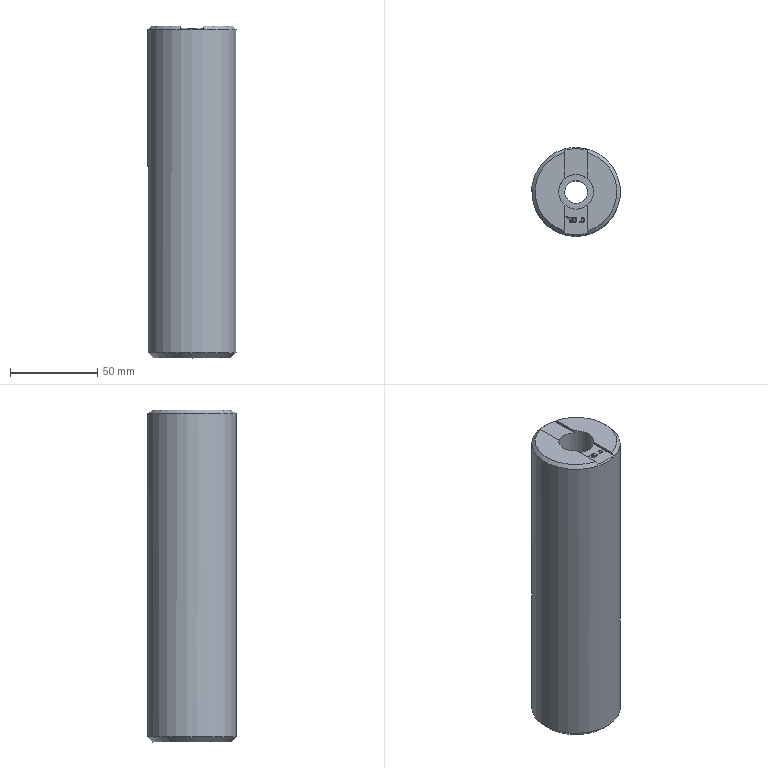Part | STEP file | 1_id1358_x_t | 1 solid | 51 faces | box 50.8 x 50.8 x 190.275 mm | volume 342596 mm3 | plane 26 | other 18 | cylinder 5 | cone 2 | commonest cylinder face diameters 468.424 x2 13 x1 20 x1 50.8 x1